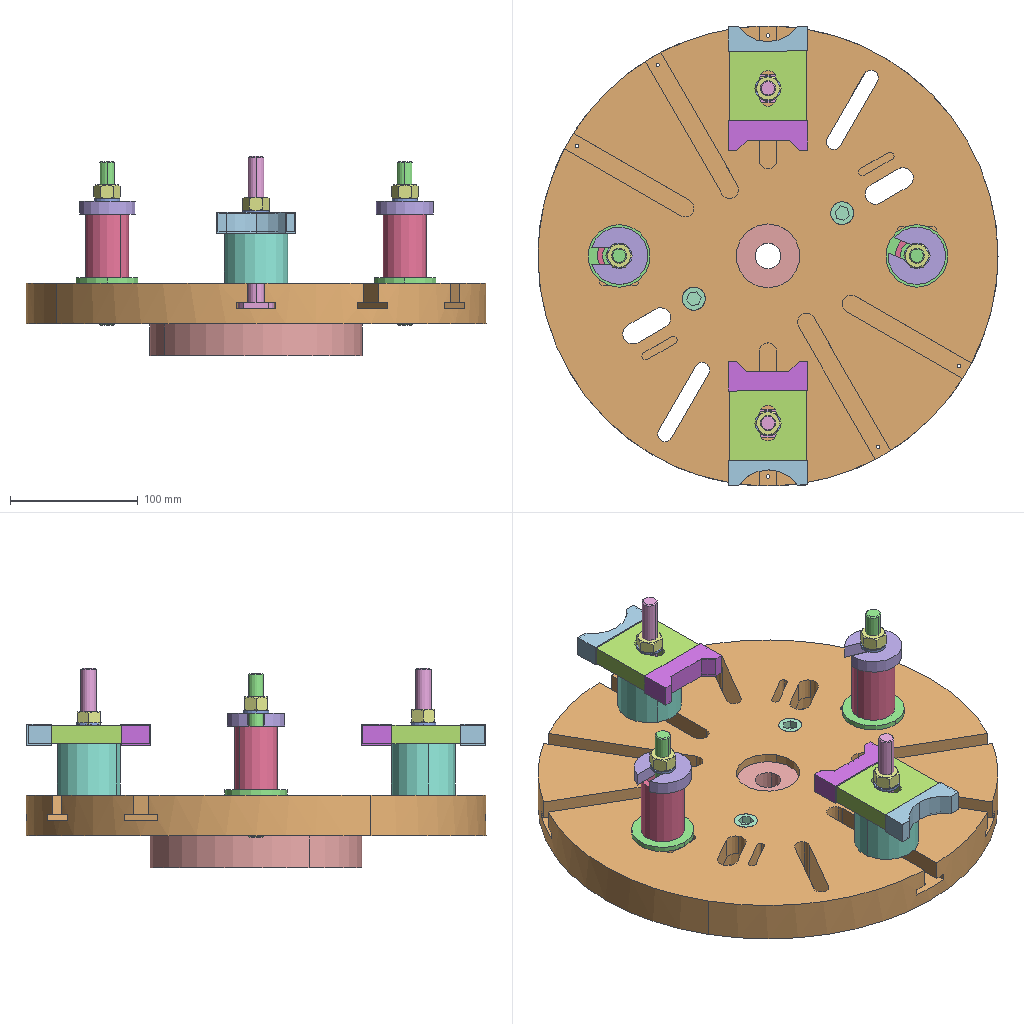Assembly | SolidWorks | 13 different items | 34 placed | box 360 x 360 x 156 mm
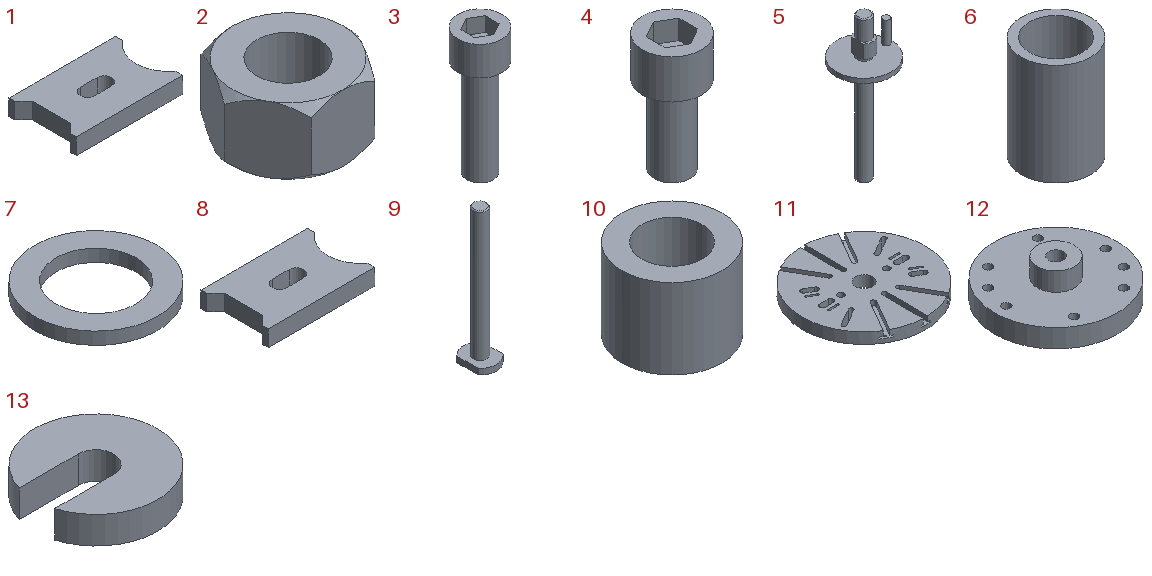Parts list (item | quantity | size | volume | features):
1 | x4 | 95 x 60 x 14.5 mm | 67299 mm3 | features ICE 2, Shell 2, Extrusion 1
2 | x6 | 20.785 x 18 x 10.8 mm | 2126 mm3 | features Extrusion 1, MirrorPattern 1, RevCutThin 1
3 | x2 | 18 x 18 x 52 mm | 6335 mm3 | features ICE 2, Extrusion 1
4 | x2 | 18 x 18 x 36 mm | 4815 mm3 | features ICE 2, Extrusion 1
5 | x2 | 49 x 49 x 128 mm | 22811 mm3 | features ICE 5, Chamfer 1, Extrusion 1
6 | x2 | 34 x 34 x 50 mm | 18850 mm3 | features Extrusion 1
7 | x6 | 20 x 20 x 2 mm | 362.854 mm3 | features Extrusion 1
8 | x2 | 95 x 60 x 14.5 mm | 67299 mm3 | features Extrusion 1
9 | x2 | 22 x 29 x 119.3 mm | 15762 mm3 | features Chamfer 1, Extrusion 1, ICE 1
10 | x2 | 50 x 50 x 40 mm | 50265 mm3 | features Extrusion 1
11 | x1 | 360 x 360 x 32 mm | 2735603 mm3 | features ICE 9, Extrusion 1
12 | x1 | 166 x 166 x 50 mm | 495390 mm3 | features ICE 5, Chamfer 1, Extrusion 1
13 | x2 | 44.041 x 45 x 10 mm | 12357 mm3 | features Extrusion 1
Mates (type | each side: item.copy, entity, surface, feature):
Concentric | 12.1 face cylinder Boss-Extrude2 | 11.1 face cylinder Boss-Extrude1
Coincident | 12.1 face plane Boss-Extrude1 | 11.1 face plane Boss-Extrude1
Coincident | 11.1 face plane Cut-Extrude4 | 9.1 face plane Boss-Extrude2
DistanceDim | 11.1 face plane Cut-Extrude4 | 9.1 plane
Coincident | 9.2 face plane Boss-Extrude2 | 11.1 face plane Cut-Extrude4
DistanceDim | 9.2 plane | 11.1 face plane Cut-Extrude5
Concentric | 9.1 face cylinder Boss-Extrude1 | 10.1 face cylinder Boss-Extrude1
Coincident | 11.1 face plane Boss-Extrude1 | 10.1 face plane Boss-Extrude1
Concentric | 9.2 face cylinder Boss-Extrude1 | 10.2 face cylinder Boss-Extrude1
Coincident | 10.2 face plane Boss-Extrude1 | 11.1 face plane Boss-Extrude1
Coincident | 10.2 face plane Boss-Extrude1 | 8.1 face plane Boss-Extrude1
Coincident | 8.2 face plane Boss-Extrude1 | 10.1 face plane Boss-Extrude1
Path | 9.2 select_type:25 | 8.1 select_type:24
Path | 9.1 select_type:25 | 8.2 select_type:24
Coincident | 8.2 face plane Boss-Extrude1 | 7.1 face plane Boss-Extrude1
Coincident | 9.1 axis | 7.1 axis
Coincident | 7.1 face plane Boss-Extrude1 | 2.1 face plane Boss-Extrude1
Coincident | 9.1 axis | 2.1 axis
Coincident | 7.2 face plane Boss-Extrude1 | 8.1 face plane Boss-Extrude1
Coincident | 7.2 axis | 9.2 axis
Coincident | 8.1 face plane Boss-Extrude1 | 2.2 face plane Boss-Extrude1
Coincident | 9.2 axis | 2.2 axis
Coincident | 8.2 face plane Boss-Extrude1 | 1.1 face plane Shell2 | 3 times
Coincident | 8.2 face plane Boss-Extrude1 | 1.2 face plane Shell1 | 2 times
Concentric | 8.2 face cylinder Boss-Extrude1 | 1.2 face cylinder Shell1
Coincident | 8.1 face plane Boss-Extrude1 | 1.3 face plane Shell1 | 2 times
Concentric | 8.1 face cylinder Boss-Extrude1 | 1.3 face cylinder Shell1
Coincident | 8.1 face plane Boss-Extrude1 | 1.4 face plane Shell2 | 3 times
Concentric | 12.1 face cylinder Cut-Extrude2 | 11.1 face cylinder Cut-Extrude1
Path | 5.1 select_type:25 | 11.1 select_type:24 | 2 times
Coincident | 11.1 face plane Boss-Extrude1 | 5.1 face plane Boss-Extrude2
Path | 5.2 select_type:25 | 11.1 select_type:24 | 2 times
Coincident | 11.1 face plane Boss-Extrude1 | 5.2 face plane Boss-Extrude2
Coincident | 5.1 face plane Boss-Extrude2 | 6.1 face plane Boss-Extrude1
Coincident | 5.1 axis | 6.1 axis
Coincident | 5.2 face plane Boss-Extrude2 | 6.2 face plane Boss-Extrude1
Coincident | 5.2 axis | 6.2 axis
Coincident | 13.1 face plane Boss-Extrude1 | 6.1 face plane Boss-Extrude1
Concentric | 13.1 face cylinder Boss-Extrude1 | 5.1 face cylinder Boss-Extrude1
Coincident | 6.2 face plane Boss-Extrude1 | 13.2 face plane Boss-Extrude1
Concentric | 5.2 face cylinder Boss-Extrude1 | 13.2 face cylinder Boss-Extrude1
Coincident | 13.1 face plane Boss-Extrude1 | 7.3 face plane Boss-Extrude1
Concentric | 5.1 face cylinder Boss-Extrude1 | 7.3 face cylinder Boss-Extrude1
Coincident | 7.4 face plane Boss-Extrude1 | 13.2 face plane Boss-Extrude1
Concentric | 7.4 face cylinder Boss-Extrude1 | 5.2 face cylinder Boss-Extrude1
Coincident | 7.4 face plane Boss-Extrude1 | 2.3 face plane Boss-Extrude1
Concentric | 5.2 face cylinder Boss-Extrude1 | 2.3 face cylinder Boss-Extrude1
Coincident | 7.3 face plane Boss-Extrude1 | 2.4 face plane Boss-Extrude1
Concentric | 5.1 face cylinder Boss-Extrude1 | 2.4 face cylinder Boss-Extrude1
Concentric | 5.1 face cylinder Boss-Extrude5 | 7.5 face cylinder Boss-Extrude1
Coincident | 11.1 face plane Cut-Extrude8 | 7.5 face plane Boss-Extrude1
Concentric | 5.1 face cylinder Boss-Extrude5 | 2.5 face cylinder Boss-Extrude1
Coincident | 2.5 face plane Boss-Extrude1 | 7.5 face plane Boss-Extrude1
Concentric | 5.2 face cylinder Boss-Extrude5 | 7.6 face cylinder Boss-Extrude1
Coincident | 11.1 face plane Cut-Extrude8 | 7.6 face plane Boss-Extrude1
Concentric | 5.2 face cylinder Boss-Extrude5 | 2.6 face cylinder Boss-Extrude1
Coincident | 7.6 face plane Boss-Extrude1 | 2.6 face plane Boss-Extrude1
Parallel | 1.1 face plane Boss-Extrude3 | 1.4 face plane Boss-Extrude3
DistanceDim | 11.1 plane | 9.2 face plane Boss-Extrude2
DistanceDim | 11.1 plane | 9.1 face plane Boss-Extrude2
Concentric | 11.1 face cylinder Cut-Extrude1 | 3.1 face cylinder Boss-Extrude1
Coincident | 11.1 face plane Boss-Extrude1 | 3.1 face plane Boss-Extrude2
Concentric | 11.1 face cylinder Cut-Extrude1 | 3.2 face cylinder Boss-Extrude1
Coincident | 11.1 face plane Boss-Extrude1 | 3.2 face plane Boss-Extrude2
Concentric | 12.1 face cylinder Cut-Extrude4 | 4.1 face cylinder Boss-Extrude1
Coincident | 12.1 face plane Boss-Extrude1 | 4.1 face plane Boss-Extrude2
Concentric | 12.1 face cylinder Cut-Extrude2 | 4.2 face cylinder Boss-Extrude1
Coincident | 12.1 face plane Boss-Extrude1 | 4.2 face plane Boss-Extrude2
Coincident | 11.1 plane | assembly plane | 2 times